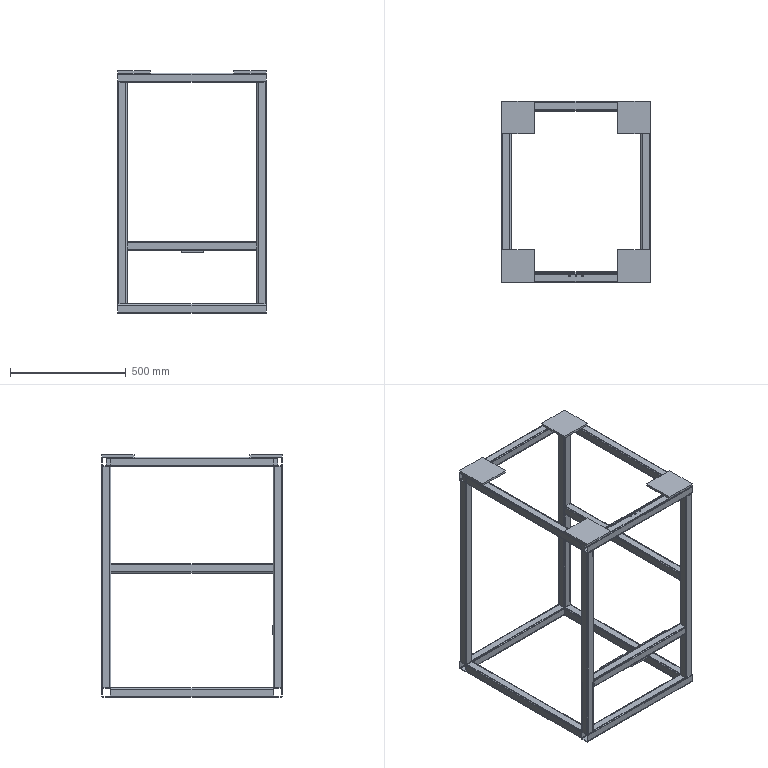Part | STEP file | PN_0029 | 21 solids | 340 faces | box 640 x 780 x 1045 mm | volume 4745237 mm3 | plane 182 | cylinder 158 | commonest cylinder face diameters 5 x64 10 x56 6.8 x38